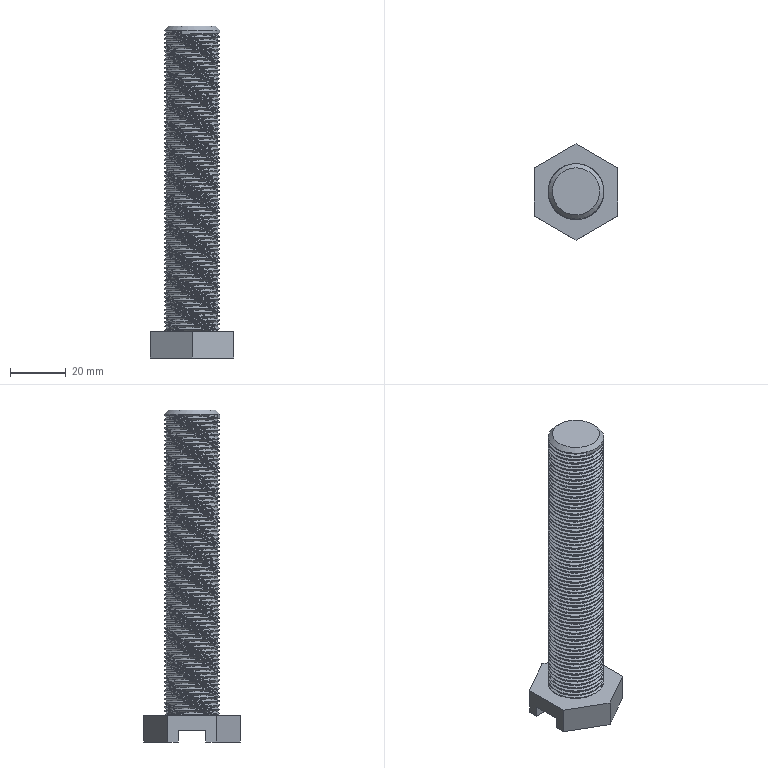Part | STEP file | YBQDJ-YB-8 | 1 solid | 19 faces | box 30 x 34.641 x 119.5 mm | volume 39653 mm3 | plane 14 | cylinder 2 | spline 2 | cone 1 | commonest cylinder face diameters 18.5 x1 20 x1